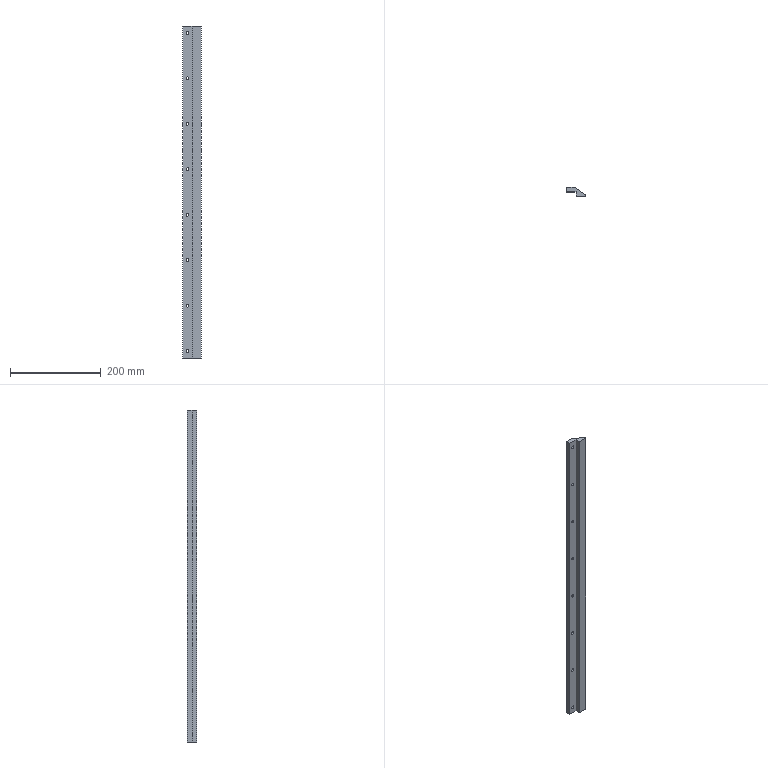Part | NX | 1 solid | 17 faces | box 40 x 20 x 730 mm | volume 284937 mm3 | plane 9 | cylinder 8 | commonest cylinder face diameters 6.2 x8
STEP:
#1=CARTESIAN_POINT('',(-20.,10.,0.));
#2=VERTEX_POINT('',#1);
#3=CARTESIAN_POINT('',(-20.,0.,0.));
#4=VERTEX_POINT('',#3);
#5=CARTESIAN_POINT('',(-20.,10.,0.));
#6=DIRECTION('',(0.,-1.,0.));
#7=VECTOR('',#6,1000.);
#8=LINE('',#5,#7);
#9=EDGE_CURVE('',#2,#4,#8,.T.);
#10=ORIENTED_EDGE('',*,*,#9,.F.);
#11=CARTESIAN_POINT('',(-20.,10.,-730.));
#12=VERTEX_POINT('',#11);
#13=CARTESIAN_POINT('',(-20.,10.,-730.));
#14=DIRECTION('',(0.,0.,1.));
#15=VECTOR('',#14,1000.);
#16=LINE('',#13,#15);
#17=EDGE_CURVE('',#12,#2,#16,.T.);
#18=ORIENTED_EDGE('',*,*,#17,.F.);
#19=CARTESIAN_POINT('',(-20.,0.,-730.));
#20=VERTEX_POINT('',#19);
#21=CARTESIAN_POINT('',(-20.,10.,-730.));
#22=DIRECTION('',(0.,-1.,0.));
#23=VECTOR('',#22,1000.);
#24=LINE('',#21,#23);
#25=EDGE_CURVE('',#12,#20,#24,.T.);
#26=ORIENTED_EDGE('',*,*,#25,.T.);
#27=CARTESIAN_POINT('',(-20.,0.,-730.));
#28=DIRECTION('',(0.,0.,1.));
#29=VECTOR('',#28,1000.);
#30=LINE('',#27,#29);
#31=EDGE_CURVE('',#20,#4,#30,.T.);
#32=ORIENTED_EDGE('',*,*,#31,.T.);
#33=EDGE_LOOP('',(#10,#18,#26,#32));
#34=FACE_BOUND('',#33,.T.);
#35=CARTESIAN_POINT('',(-20.,10.,-730.));
#36=DIRECTION('',(-1.,0.,0.));
#37=DIRECTION('',(0.,0.,1.));
#38=AXIS2_PLACEMENT_3D('',#35,#36,#37);
#39=PLANE('',#38);
#40=ADVANCED_FACE('',(#34),#39,.T.);
#41=CARTESIAN_POINT('',(-6.9,0.,-15.));
#42=VERTEX_POINT('',#41);
#43=CARTESIAN_POINT('',(-10.,0.,-15.));
#44=DIRECTION('',(0.,-1.,0.));
#45=DIRECTION('',(1.,0.,0.));
#46=AXIS2_PLACEMENT_3D('',#43,#44,#45);
#47=CIRCLE('',#46,3.1);
#48=EDGE_CURVE('',#42,#42,#47,.T.);
#49=ORIENTED_EDGE('',*,*,#48,.F.);
#50=EDGE_LOOP('',(#49));
#51=FACE_BOUND('',#50,.T.);
#52=CARTESIAN_POINT('',(-6.9,0.,-115.));
#53=VERTEX_POINT('',#52);
#54=CARTESIAN_POINT('',(-10.,0.,-115.));
#55=DIRECTION('',(0.,-1.,0.));
#56=DIRECTION('',(1.,0.,0.));
#57=AXIS2_PLACEMENT_3D('',#54,#55,#56);
#58=CIRCLE('',#57,3.1);
#59=EDGE_CURVE('',#53,#53,#58,.T.);
#60=ORIENTED_EDGE('',*,*,#59,.F.);
#61=EDGE_LOOP('',(#60));
#62=FACE_BOUND('',#61,.T.);
#63=CARTESIAN_POINT('',(-6.9,0.,-215.));
#64=VERTEX_POINT('',#63);
#65=CARTESIAN_POINT('',(-10.,0.,-215.));
#66=DIRECTION('',(0.,-1.,0.));
#67=DIRECTION('',(1.,0.,0.));
#68=AXIS2_PLACEMENT_3D('',#65,#66,#67);
#69=CIRCLE('',#68,3.1);
#70=EDGE_CURVE('',#64,#64,#69,.T.);
#71=ORIENTED_EDGE('',*,*,#70,.F.);
#72=EDGE_LOOP('',(#71));
#73=FACE_BOUND('',#72,.T.);
#74=CARTESIAN_POINT('',(-6.9,0.,-315.));
#75=VERTEX_POINT('',#74);
#76=CARTESIAN_POINT('',(-10.,0.,-315.));
#77=DIRECTION('',(0.,-1.,0.));
#78=DIRECTION('',(1.,0.,0.));
#79=AXIS2_PLACEMENT_3D('',#76,#77,#78);
#80=CIRCLE('',#79,3.1);
#81=EDGE_CURVE('',#75,#75,#80,.T.);
#82=ORIENTED_EDGE('',*,*,#81,.F.);
#83=EDGE_LOOP('',(#82));
#84=FACE_BOUND('',#83,.T.);
#85=CARTESIAN_POINT('',(-6.9,0.,-415.));
#86=VERTEX_POINT('',#85);
#87=CARTESIAN_POINT('',(-10.,0.,-415.));
#88=DIRECTION('',(0.,-1.,0.));
#89=DIRECTION('',(1.,0.,0.));
#90=AXIS2_PLACEMENT_3D('',#87,#88,#89);
#91=CIRCLE('',#90,3.1);
#92=EDGE_CURVE('',#86,#86,#91,.T.);
#93=ORIENTED_EDGE('',*,*,#92,.F.);
#94=EDGE_LOOP('',(#93));
#95=FACE_BOUND('',#94,.T.);
#96=CARTESIAN_POINT('',(-6.9,0.,-515.));
#97=VERTEX_POINT('',#96);
#98=CARTESIAN_POINT('',(-10.,0.,-515.));
#99=DIRECTION('',(0.,-1.,0.));
#100=DIRECTION('',(1.,0.,0.));
#101=AXIS2_PLACEMENT_3D('',#98,#99,#100);
#102=CIRCLE('',#101,3.1);
#103=EDGE_CURVE('',#97,#97,#102,.T.);
#104=ORIENTED_EDGE('',*,*,#103,.F.);
#105=EDGE_LOOP('',(#104));
#106=FACE_BOUND('',#105,.T.);
#107=CARTESIAN_POINT('',(-6.9,0.,-615.));
#108=VERTEX_POINT('',#107);
#109=CARTESIAN_POINT('',(-10.,0.,-615.));
#110=DIRECTION('',(0.,-1.,0.));
#111=DIRECTION('',(1.,0.,0.));
#112=AXIS2_PLACEMENT_3D('',#109,#110,#111);
#113=CIRCLE('',#112,3.1);
#114=EDGE_CURVE('',#108,#108,#113,.T.);
#115=ORIENTED_EDGE('',*,*,#114,.F.);
#116=EDGE_LOOP('',(#115));
#117=FACE_BOUND('',#116,.T.);
#118=CARTESIAN_POINT('',(-6.9,0.,-715.));
#119=VERTEX_POINT('',#118);
#120=CARTESIAN_POINT('',(-10.,0.,-715.));
#121=DIRECTION('',(0.,-1.,0.));
#122=DIRECTION('',(1.,0.,0.));
#123=AXIS2_PLACEMENT_3D('',#120,#121,#122);
#124=CIRCLE('',#123,3.1);
#125=EDGE_CURVE('',#119,#119,#124,.T.);
#126=ORIENTED_EDGE('',*,*,#125,.F.);
#127=EDGE_LOOP('',(#126));
#128=FACE_BOUND('',#127,.T.);
#129=CARTESIAN_POINT('',(0.,0.,0.));
#130=VERTEX_POINT('',#129);
#131=CARTESIAN_POINT('',(-20.,0.,0.));
#132=DIRECTION('',(1.,0.,0.));
#133=VECTOR('',#132,1000.);
#134=LINE('',#131,#133);
#135=EDGE_CURVE('',#4,#130,#134,.T.);
#136=ORIENTED_EDGE('',*,*,#135,.F.);
#137=ORIENTED_EDGE('',*,*,#31,.F.);
#138=CARTESIAN_POINT('',(0.,0.,-730.));
#139=VERTEX_POINT('',#138);
#140=CARTESIAN_POINT('',(-20.,0.,-730.));
#141=DIRECTION('',(1.,0.,0.));
#142=VECTOR('',#141,1000.);
#143=LINE('',#140,#142);
#144=EDGE_CURVE('',#20,#139,#143,.T.);
#145=ORIENTED_EDGE('',*,*,#144,.T.);
#146=CARTESIAN_POINT('',(0.,0.,-730.));
#147=DIRECTION('',(0.,0.,1.));
#148=VECTOR('',#147,1000.);
#149=LINE('',#146,#148);
#150=EDGE_CURVE('',#139,#130,#149,.T.);
#151=ORIENTED_EDGE('',*,*,#150,.T.);
#152=EDGE_LOOP('',(#136,#137,#145,#151));
#153=FACE_BOUND('',#152,.T.);
#154=CARTESIAN_POINT('',(-20.,0.,-730.));
#155=DIRECTION('',(0.,-1.,0.));
#156=DIRECTION('',(1.,0.,0.));
#157=AXIS2_PLACEMENT_3D('',#154,#155,#156);
#158=PLANE('',#157);
#159=ADVANCED_FACE('',(#51,#62,#73,#84,#95,#106,#117,#128,#153),#158,.T.);
#160=CARTESIAN_POINT('',(0.,-10.,0.));
#161=VERTEX_POINT('',#160);
#162=CARTESIAN_POINT('',(0.,0.,0.));
#163=DIRECTION('',(0.,-1.,0.));
#164=VECTOR('',#163,1000.);
#165=LINE('',#162,#164);
#166=EDGE_CURVE('',#130,#161,#165,.T.);
#167=ORIENTED_EDGE('',*,*,#166,.F.);
#168=ORIENTED_EDGE('',*,*,#150,.F.);
#169=CARTESIAN_POINT('',(0.,-10.,-730.));
#170=VERTEX_POINT('',#169);
#171=CARTESIAN_POINT('',(0.,0.,-730.));
#172=DIRECTION('',(0.,-1.,0.));
#173=VECTOR('',#172,1000.);
#174=LINE('',#171,#173);
#175=EDGE_CURVE('',#139,#170,#174,.T.);
#176=ORIENTED_EDGE('',*,*,#175,.T.);
#177=CARTESIAN_POINT('',(0.,-10.,-730.));
#178=DIRECTION('',(0.,0.,1.));
#179=VECTOR('',#178,1000.);
#180=LINE('',#177,#179);
#181=EDGE_CURVE('',#170,#161,#180,.T.);
#182=ORIENTED_EDGE('',*,*,#181,.T.);
#183=EDGE_LOOP('',(#167,#168,#176,#182));
#184=FACE_BOUND('',#183,.T.);
#185=CARTESIAN_POINT('',(0.,0.,-730.));
#186=DIRECTION('',(-1.,0.,0.));
#187=DIRECTION('',(0.,-1.,0.));
#188=AXIS2_PLACEMENT_3D('',#185,#186,#187);
#189=PLANE('',#188);
#190=ADVANCED_FACE('',(#184),#189,.T.);
#191=CARTESIAN_POINT('',(20.,-10.,0.));
#192=VERTEX_POINT('',#191);
#193=CARTESIAN_POINT('',(0.,-10.,0.));
#194=DIRECTION('',(1.,0.,0.));
#195=VECTOR('',#194,1000.);
#196=LINE('',#193,#195);
#197=EDGE_CURVE('',#161,#192,#196,.T.);
#198=ORIENTED_EDGE('',*,*,#197,.F.);
#199=ORIENTED_EDGE('',*,*,#181,.F.);
#200=CARTESIAN_POINT('',(20.,-10.,-730.));
#201=VERTEX_POINT('',#200);
#202=CARTESIAN_POINT('',(0.,-10.,-730.));
#203=DIRECTION('',(1.,0.,0.));
#204=VECTOR('',#203,1000.);
#205=LINE('',#202,#204);
#206=EDGE_CURVE('',#170,#201,#205,.T.);
#207=ORIENTED_EDGE('',*,*,#206,.T.);
#208=CARTESIAN_POINT('',(20.,-10.,-730.));
#209=DIRECTION('',(0.,0.,1.));
#210=VECTOR('',#209,1000.);
#211=LINE('',#208,#210);
#212=EDGE_CURVE('',#201,#192,#211,.T.);
#213=ORIENTED_EDGE('',*,*,#212,.T.);
#214=EDGE_LOOP('',(#198,#199,#207,#213));
#215=FACE_BOUND('',#214,.T.);
#216=CARTESIAN_POINT('',(0.,-10.,-730.));
#217=DIRECTION('',(0.,-1.,0.));
#218=DIRECTION('',(1.,0.,0.));
#219=AXIS2_PLACEMENT_3D('',#216,#217,#218);
#220=PLANE('',#219);
#221=ADVANCED_FACE('',(#215),#220,.T.);
#222=CARTESIAN_POINT('',(20.,-7.,0.));
#223=VERTEX_POINT('',#222);
#224=CARTESIAN_POINT('',(20.,-10.,0.));
#225=DIRECTION('',(0.,1.,0.));
#226=VECTOR('',#225,1000.);
#227=LINE('',#224,#226);
#228=EDGE_CURVE('',#192,#223,#227,.T.);
#229=ORIENTED_EDGE('',*,*,#228,.F.);
#230=ORIENTED_EDGE('',*,*,#212,.F.);
#231=CARTESIAN_POINT('',(20.,-7.,-730.));
#232=VERTEX_POINT('',#231);
#233=CARTESIAN_POINT('',(20.,-10.,-730.));
#234=DIRECTION('',(0.,1.,0.));
#235=VECTOR('',#234,1000.);
#236=LINE('',#233,#235);
#237=EDGE_CURVE('',#201,#232,#236,.T.);
#238=ORIENTED_EDGE('',*,*,#237,.T.);
#239=CARTESIAN_POINT('',(20.,-7.,-730.));
#240=DIRECTION('',(0.,0.,1.));
#241=VECTOR('',#240,1000.);
#242=LINE('',#239,#241);
#243=EDGE_CURVE('',#232,#223,#242,.T.);
#244=ORIENTED_EDGE('',*,*,#243,.T.);
#245=EDGE_LOOP('',(#229,#230,#238,#244));
#246=FACE_BOUND('',#245,.T.);
#247=CARTESIAN_POINT('',(20.,-10.,-730.));
#248=DIRECTION('',(1.,0.,0.));
#249=DIRECTION('',(0.,0.,-1.));
#250=AXIS2_PLACEMENT_3D('',#247,#248,#249);
#251=PLANE('',#250);
#252=ADVANCED_FACE('',(#246),#251,.T.);
#253=CARTESIAN_POINT('',(-4.279,10.,0.));
#254=VERTEX_POINT('',#253);
#255=CARTESIAN_POINT('',(20.,-7.,0.));
#256=DIRECTION('',(-0.8192,0.5736,0.));
#257=VECTOR('',#256,1000.);
#258=LINE('',#255,#257);
#259=EDGE_CURVE('',#223,#254,#258,.T.);
#260=ORIENTED_EDGE('',*,*,#259,.F.);
#261=ORIENTED_EDGE('',*,*,#243,.F.);
#262=CARTESIAN_POINT('',(-4.279,10.,-730.));
#263=VERTEX_POINT('',#262);
#264=CARTESIAN_POINT('',(20.,-7.,-730.));
#265=DIRECTION('',(-0.8192,0.5736,0.));
#266=VECTOR('',#265,1000.);
#267=LINE('',#264,#266);
#268=EDGE_CURVE('',#232,#263,#267,.T.);
#269=ORIENTED_EDGE('',*,*,#268,.T.);
#270=CARTESIAN_POINT('',(-4.279,10.,-730.));
#271=DIRECTION('',(0.,0.,1.));
#272=VECTOR('',#271,1000.);
#273=LINE('',#270,#272);
#274=EDGE_CURVE('',#263,#254,#273,.T.);
#275=ORIENTED_EDGE('',*,*,#274,.T.);
#276=EDGE_LOOP('',(#260,#261,#269,#275));
#277=FACE_BOUND('',#276,.T.);
#278=CARTESIAN_POINT('',(20.,-7.,-730.));
#279=DIRECTION('',(0.5736,0.8192,0.));
#280=DIRECTION('',(-0.8192,0.5736,0.));
#281=AXIS2_PLACEMENT_3D('',#278,#279,#280);
#282=PLANE('',#281);
#283=ADVANCED_FACE('',(#277),#282,.T.);
#284=CARTESIAN_POINT('',(-10.,10.,-11.9));
#285=VERTEX_POINT('',#284);
#286=CARTESIAN_POINT('',(-10.,10.,-15.));
#287=DIRECTION('',(0.,1.,0.));
#288=DIRECTION('',(0.,0.,1.));
#289=AXIS2_PLACEMENT_3D('',#286,#287,#288);
#290=CIRCLE('',#289,3.1);
#291=EDGE_CURVE('',#285,#285,#290,.T.);
#292=ORIENTED_EDGE('',*,*,#291,.F.);
#293=EDGE_LOOP('',(#292));
#294=FACE_BOUND('',#293,.T.);
#295=CARTESIAN_POINT('',(-10.,10.,-111.9));
#296=VERTEX_POINT('',#295);
#297=CARTESIAN_POINT('',(-10.,10.,-115.));
#298=DIRECTION('',(0.,1.,0.));
#299=DIRECTION('',(0.,0.,1.));
#300=AXIS2_PLACEMENT_3D('',#297,#298,#299);
#301=CIRCLE('',#300,3.1);
#302=EDGE_CURVE('',#296,#296,#301,.T.);
#303=ORIENTED_EDGE('',*,*,#302,.F.);
#304=EDGE_LOOP('',(#303));
#305=FACE_BOUND('',#304,.T.);
#306=CARTESIAN_POINT('',(-10.,10.,-211.9));
#307=VERTEX_POINT('',#306);
#308=CARTESIAN_POINT('',(-10.,10.,-215.));
#309=DIRECTION('',(0.,1.,0.));
#310=DIRECTION('',(0.,0.,1.));
#311=AXIS2_PLACEMENT_3D('',#308,#309,#310);
#312=CIRCLE('',#311,3.1);
#313=EDGE_CURVE('',#307,#307,#312,.T.);
#314=ORIENTED_EDGE('',*,*,#313,.F.);
#315=EDGE_LOOP('',(#314));
#316=FACE_BOUND('',#315,.T.);
#317=CARTESIAN_POINT('',(-10.,10.,-311.9));
#318=VERTEX_POINT('',#317);
#319=CARTESIAN_POINT('',(-10.,10.,-315.));
#320=DIRECTION('',(0.,1.,0.));
#321=DIRECTION('',(0.,0.,1.));
#322=AXIS2_PLACEMENT_3D('',#319,#320,#321);
#323=CIRCLE('',#322,3.1);
#324=EDGE_CURVE('',#318,#318,#323,.T.);
#325=ORIENTED_EDGE('',*,*,#324,.F.);
#326=EDGE_LOOP('',(#325));
#327=FACE_BOUND('',#326,.T.);
#328=CARTESIAN_POINT('',(-10.,10.,-411.9));
#329=VERTEX_POINT('',#328);
#330=CARTESIAN_POINT('',(-10.,10.,-415.));
#331=DIRECTION('',(0.,1.,0.));
#332=DIRECTION('',(0.,0.,1.));
#333=AXIS2_PLACEMENT_3D('',#330,#331,#332);
#334=CIRCLE('',#333,3.1);
#335=EDGE_CURVE('',#329,#329,#334,.T.);
#336=ORIENTED_EDGE('',*,*,#335,.F.);
#337=EDGE_LOOP('',(#336));
#338=FACE_BOUND('',#337,.T.);
#339=CARTESIAN_POINT('',(-10.,10.,-511.9));
#340=VERTEX_POINT('',#339);
#341=CARTESIAN_POINT('',(-10.,10.,-515.));
#342=DIRECTION('',(0.,1.,0.));
#343=DIRECTION('',(0.,0.,1.));
#344=AXIS2_PLACEMENT_3D('',#341,#342,#343);
#345=CIRCLE('',#344,3.1);
#346=EDGE_CURVE('',#340,#340,#345,.T.);
#347=ORIENTED_EDGE('',*,*,#346,.F.);
#348=EDGE_LOOP('',(#347));
#349=FACE_BOUND('',#348,.T.);
#350=CARTESIAN_POINT('',(-10.,10.,-611.9));
#351=VERTEX_POINT('',#350);
#352=CARTESIAN_POINT('',(-10.,10.,-615.));
#353=DIRECTION('',(0.,1.,0.));
#354=DIRECTION('',(0.,0.,1.));
#355=AXIS2_PLACEMENT_3D('',#352,#353,#354);
#356=CIRCLE('',#355,3.1);
#357=EDGE_CURVE('',#351,#351,#356,.T.);
#358=ORIENTED_EDGE('',*,*,#357,.F.);
#359=EDGE_LOOP('',(#358));
#360=FACE_BOUND('',#359,.T.);
#361=CARTESIAN_POINT('',(-10.,10.,-711.9));
#362=VERTEX_POINT('',#361);
#363=CARTESIAN_POINT('',(-10.,10.,-715.));
#364=DIRECTION('',(0.,1.,0.));
#365=DIRECTION('',(0.,0.,1.));
#366=AXIS2_PLACEMENT_3D('',#363,#364,#365);
#367=CIRCLE('',#366,3.1);
#368=EDGE_CURVE('',#362,#362,#367,.T.);
#369=ORIENTED_EDGE('',*,*,#368,.F.);
#370=EDGE_LOOP('',(#369));
#371=FACE_BOUND('',#370,.T.);
#372=CARTESIAN_POINT('',(-4.279,10.,0.));
#373=DIRECTION('',(-1.,0.,0.));
#374=VECTOR('',#373,1000.);
#375=LINE('',#372,#374);
#376=EDGE_CURVE('',#254,#2,#375,.T.);
#377=ORIENTED_EDGE('',*,*,#376,.F.);
#378=ORIENTED_EDGE('',*,*,#274,.F.);
#379=CARTESIAN_POINT('',(-4.279,10.,-730.));
#380=DIRECTION('',(-1.,0.,0.));
#381=VECTOR('',#380,1000.);
#382=LINE('',#379,#381);
#383=EDGE_CURVE('',#263,#12,#382,.T.);
#384=ORIENTED_EDGE('',*,*,#383,.T.);
#385=ORIENTED_EDGE('',*,*,#17,.T.);
#386=EDGE_LOOP('',(#377,#378,#384,#385));
#387=FACE_BOUND('',#386,.T.);
#388=CARTESIAN_POINT('',(-4.279,10.,-730.));
#389=DIRECTION('',(0.,1.,0.));
#390=DIRECTION('',(-1.,0.,0.));
#391=AXIS2_PLACEMENT_3D('',#388,#389,#390);
#392=PLANE('',#391);
#393=ADVANCED_FACE('',(#294,#305,#316,#327,#338,#349,#360,#371,#387),#392,.T.);
#394=ORIENTED_EDGE('',*,*,#25,.F.);
#395=ORIENTED_EDGE('',*,*,#383,.F.);
#396=ORIENTED_EDGE('',*,*,#268,.F.);
#397=ORIENTED_EDGE('',*,*,#237,.F.);
#398=ORIENTED_EDGE('',*,*,#206,.F.);
#399=ORIENTED_EDGE('',*,*,#175,.F.);
#400=ORIENTED_EDGE('',*,*,#144,.F.);
#401=EDGE_LOOP('',(#394,#395,#396,#397,#398,#399,#400));
#402=FACE_BOUND('',#401,.T.);
#403=CARTESIAN_POINT('',(0.,0.,-730.));
#404=DIRECTION('',(0.,0.,1.));
#405=DIRECTION('',(1.,0.,0.));
#406=AXIS2_PLACEMENT_3D('',#403,#404,#405);
#407=PLANE('',#406);
#408=ADVANCED_FACE('',(#402),#407,.F.);
#409=ORIENTED_EDGE('',*,*,#9,.T.);
#410=ORIENTED_EDGE('',*,*,#135,.T.);
#411=ORIENTED_EDGE('',*,*,#166,.T.);
#412=ORIENTED_EDGE('',*,*,#197,.T.);
#413=ORIENTED_EDGE('',*,*,#228,.T.);
#414=ORIENTED_EDGE('',*,*,#259,.T.);
#415=ORIENTED_EDGE('',*,*,#376,.T.);
#416=EDGE_LOOP('',(#409,#410,#411,#412,#413,#414,#415));
#417=FACE_BOUND('',#416,.T.);
#418=CARTESIAN_POINT('',(0.,0.,0.));
#419=DIRECTION('',(0.,0.,1.));
#420=DIRECTION('',(1.,0.,0.));
#421=AXIS2_PLACEMENT_3D('',#418,#419,#420);
#422=PLANE('',#421);
#423=ADVANCED_FACE('',(#417),#422,.T.);
#424=ORIENTED_EDGE('',*,*,#125,.T.);
#425=EDGE_LOOP('',(#424));
#426=FACE_BOUND('',#425,.T.);
#427=ORIENTED_EDGE('',*,*,#368,.T.);
#428=EDGE_LOOP('',(#427));
#429=FACE_BOUND('',#428,.T.);
#430=CARTESIAN_POINT('',(-10.,-10.,-715.));
#431=DIRECTION('',(0.,1.,0.));
#432=DIRECTION('',(-1.,0.,0.));
#433=AXIS2_PLACEMENT_3D('',#430,#431,#432);
#434=CYLINDRICAL_SURFACE('',#433,3.1);
#435=ADVANCED_FACE('',(#426,#429),#434,.F.);
#436=ORIENTED_EDGE('',*,*,#114,.T.);
#437=EDGE_LOOP('',(#436));
#438=FACE_BOUND('',#437,.T.);
#439=ORIENTED_EDGE('',*,*,#357,.T.);
#440=EDGE_LOOP('',(#439));
#441=FACE_BOUND('',#440,.T.);
#442=CARTESIAN_POINT('',(-10.,-10.,-615.));
#443=DIRECTION('',(0.,1.,0.));
#444=DIRECTION('',(-1.,0.,0.));
#445=AXIS2_PLACEMENT_3D('',#442,#443,#444);
#446=CYLINDRICAL_SURFACE('',#445,3.1);
#447=ADVANCED_FACE('',(#438,#441),#446,.F.);
#448=ORIENTED_EDGE('',*,*,#103,.T.);
#449=EDGE_LOOP('',(#448));
#450=FACE_BOUND('',#449,.T.);
#451=ORIENTED_EDGE('',*,*,#346,.T.);
#452=EDGE_LOOP('',(#451));
#453=FACE_BOUND('',#452,.T.);
#454=CARTESIAN_POINT('',(-10.,-10.,-515.));
#455=DIRECTION('',(0.,1.,0.));
#456=DIRECTION('',(-1.,0.,0.));
#457=AXIS2_PLACEMENT_3D('',#454,#455,#456);
#458=CYLINDRICAL_SURFACE('',#457,3.1);
#459=ADVANCED_FACE('',(#450,#453),#458,.F.);
#460=ORIENTED_EDGE('',*,*,#92,.T.);
#461=EDGE_LOOP('',(#460));
#462=FACE_BOUND('',#461,.T.);
#463=ORIENTED_EDGE('',*,*,#335,.T.);
#464=EDGE_LOOP('',(#463));
#465=FACE_BOUND('',#464,.T.);
#466=CARTESIAN_POINT('',(-10.,-10.,-415.));
#467=DIRECTION('',(0.,1.,0.));
#468=DIRECTION('',(-1.,0.,0.));
#469=AXIS2_PLACEMENT_3D('',#466,#467,#468);
#470=CYLINDRICAL_SURFACE('',#469,3.1);
#471=ADVANCED_FACE('',(#462,#465),#470,.F.);
#472=ORIENTED_EDGE('',*,*,#81,.T.);
#473=EDGE_LOOP('',(#472));
#474=FACE_BOUND('',#473,.T.);
#475=ORIENTED_EDGE('',*,*,#324,.T.);
#476=EDGE_LOOP('',(#475));
#477=FACE_BOUND('',#476,.T.);
#478=CARTESIAN_POINT('',(-10.,-10.,-315.));
#479=DIRECTION('',(0.,1.,0.));
#480=DIRECTION('',(-1.,0.,0.));
#481=AXIS2_PLACEMENT_3D('',#478,#479,#480);
#482=CYLINDRICAL_SURFACE('',#481,3.1);
#483=ADVANCED_FACE('',(#474,#477),#482,.F.);
#484=ORIENTED_EDGE('',*,*,#70,.T.);
#485=EDGE_LOOP('',(#484));
#486=FACE_BOUND('',#485,.T.);
#487=ORIENTED_EDGE('',*,*,#313,.T.);
#488=EDGE_LOOP('',(#487));
#489=FACE_BOUND('',#488,.T.);
#490=CARTESIAN_POINT('',(-10.,-10.,-215.));
#491=DIRECTION('',(0.,1.,0.));
#492=DIRECTION('',(-1.,0.,0.));
#493=AXIS2_PLACEMENT_3D('',#490,#491,#492);
#494=CYLINDRICAL_SURFACE('',#493,3.1);
#495=ADVANCED_FACE('',(#486,#489),#494,.F.);
#496=ORIENTED_EDGE('',*,*,#59,.T.);
#497=EDGE_LOOP('',(#496));
#498=FACE_BOUND('',#497,.T.);
#499=ORIENTED_EDGE('',*,*,#302,.T.);
#500=EDGE_LOOP('',(#499));
#501=FACE_BOUND('',#500,.T.);
#502=CARTESIAN_POINT('',(-10.,-10.,-115.));
#503=DIRECTION('',(0.,1.,0.));
#504=DIRECTION('',(-1.,0.,0.));
#505=AXIS2_PLACEMENT_3D('',#502,#503,#504);
#506=CYLINDRICAL_SURFACE('',#505,3.1);
#507=ADVANCED_FACE('',(#498,#501),#506,.F.);
#508=ORIENTED_EDGE('',*,*,#48,.T.);
#509=EDGE_LOOP('',(#508));
#510=FACE_BOUND('',#509,.T.);
#511=ORIENTED_EDGE('',*,*,#291,.T.);
#512=EDGE_LOOP('',(#511));
#513=FACE_BOUND('',#512,.T.);
#514=CARTESIAN_POINT('',(-10.,-10.,-15.));
#515=DIRECTION('',(0.,1.,0.));
#516=DIRECTION('',(-1.,0.,0.));
#517=AXIS2_PLACEMENT_3D('',#514,#515,#516);
#518=CYLINDRICAL_SURFACE('',#517,3.1);
#519=ADVANCED_FACE('',(#510,#513),#518,.F.);
#520=CLOSED_SHELL('',(#40,#159,#190,#221,#252,#283,#393,#408,#423,#435,#447,#459,#471,#483,#495,#507,#519));
#521=MANIFOLD_SOLID_BREP('',#520);
#522=(LENGTH_UNIT()NAMED_UNIT(*)SI_UNIT(.MILLI.,.METRE.));
#523=UNCERTAINTY_MEASURE_WITH_UNIT(LENGTH_MEASURE(0.00001),#522,'','');
#524=(NAMED_UNIT(*)PLANE_ANGLE_UNIT()SI_UNIT($,.RADIAN.));
#525=(NAMED_UNIT(*)SI_UNIT($,.STERADIAN.)SOLID_ANGLE_UNIT());
#526=(GEOMETRIC_REPRESENTATION_CONTEXT(3)GLOBAL_UNCERTAINTY_ASSIGNED_CONTEXT((#523))GLOBAL_UNIT_ASSIGNED_CONTEXT((#522,#524,#525))REPRESENTATION_CONTEXT('',''));
#527=ADVANCED_BREP_SHAPE_REPRESENTATION('',(#521),#526);